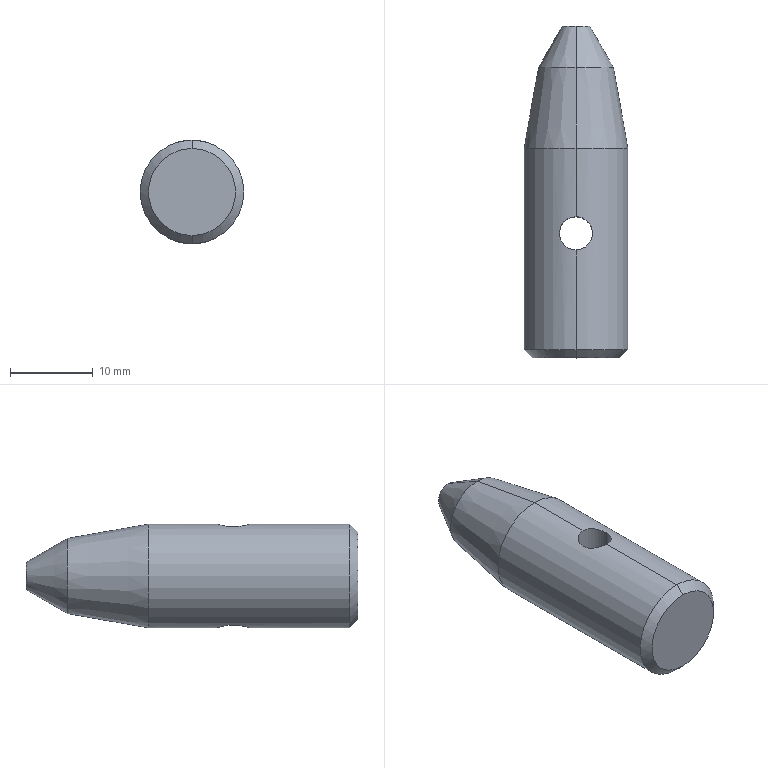Part | STEP file | PN_0055 | 1 solid | 12 faces | box 12.5 x 40 x 12.5 mm | volume 3984 mm3 | cone 6 | cylinder 4 | plane 2 | commonest cylinder face diameters 4 x2 12.5 x2